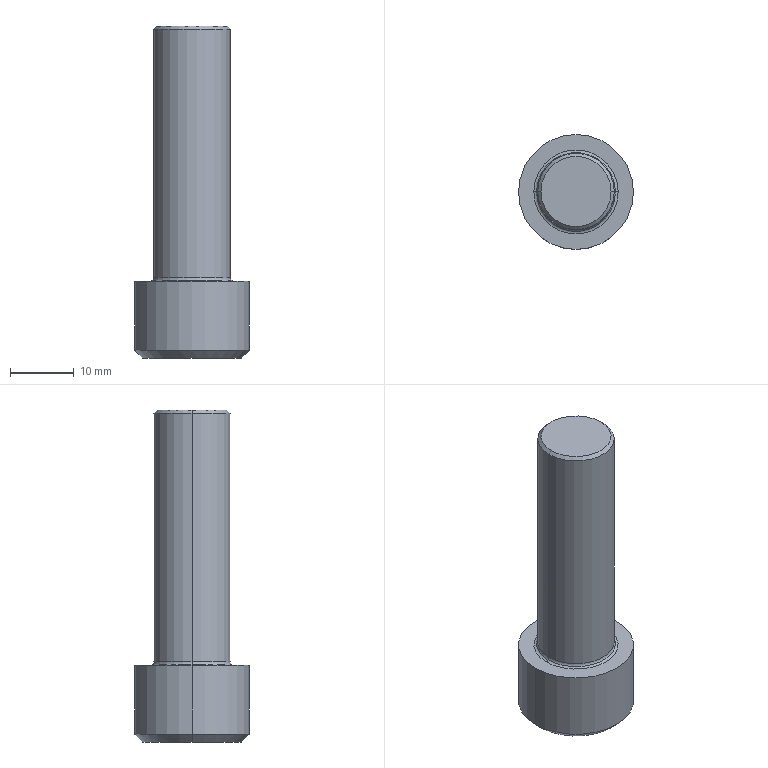Part | Creo | 1 solid | 23 faces | box 18 x 18 x 52 mm | volume 6904 mm3 | plane 9 | cone 6 | cylinder 4 | torus 4 | commonest cylinder face diameters 12 x2 18 x2
STEP:
#1=CARTESIAN_POINT('',(-0.7735,-90.005,-358.));
#2=VERTEX_POINT('',#1);
#3=CARTESIAN_POINT('',(2.113,-85.005,-358.));
#4=VERTEX_POINT('',#3);
#5=CARTESIAN_POINT('',(-0.7735,-90.005,-358.));
#6=CARTESIAN_POINT('',(-0.6388,-89.771,-357.922));
#7=CARTESIAN_POINT('',(-0.3685,-89.303,-357.782));
#8=CARTESIAN_POINT('',(0.04278,-88.591,-357.631));
#9=CARTESIAN_POINT('',(0.4589,-87.87,-357.55));
#10=CARTESIAN_POINT('',(0.8794,-87.142,-357.55));
#11=CARTESIAN_POINT('',(1.296,-86.42,-357.631));
#12=CARTESIAN_POINT('',(1.707,-85.709,-357.782));
#13=CARTESIAN_POINT('',(1.978,-85.239,-357.922));
#14=CARTESIAN_POINT('',(2.113,-85.005,-358.));
#15=B_SPLINE_CURVE_WITH_KNOTS('',3,(#5,#6,#7,#8,#9,#10,#11,#12,#13,#14),.UNSPECIFIED.,.F.,.F.,(4,1,1,1,1,1,1,4),(0.,0.1429,0.2857,0.4286,0.5714,0.7143,0.8571,1.),.UNSPECIFIED.);
#16=EDGE_CURVE('',#2,#4,#15,.T.);
#17=ORIENTED_EDGE('',*,*,#16,.F.);
#18=CARTESIAN_POINT('',(5.,-90.005,-354.667));
#19=VERTEX_POINT('',#18);
#20=CARTESIAN_POINT('',(5.,-90.005,-354.667));
#21=DIRECTION('',(-0.866,0.,-0.5));
#22=VECTOR('',#21,6.667);
#23=LINE('',#20,#22);
#24=EDGE_CURVE('',#19,#2,#23,.T.);
#25=ORIENTED_EDGE('',*,*,#24,.F.);
#26=CARTESIAN_POINT('',(10.774,-90.005,-358.));
#27=VERTEX_POINT('',#26);
#28=CARTESIAN_POINT('',(5.,-90.005,-354.667));
#29=DIRECTION('',(0.866,0.,-0.5));
#30=VECTOR('',#29,6.667);
#31=LINE('',#28,#30);
#32=EDGE_CURVE('',#19,#27,#31,.T.);
#33=ORIENTED_EDGE('',*,*,#32,.T.);
#34=CARTESIAN_POINT('',(7.887,-85.005,-358.));
#35=VERTEX_POINT('',#34);
#36=CARTESIAN_POINT('',(7.887,-85.005,-358.));
#37=CARTESIAN_POINT('',(8.021,-85.238,-357.922));
#38=CARTESIAN_POINT('',(8.292,-85.706,-357.782));
#39=CARTESIAN_POINT('',(8.703,-86.419,-357.631));
#40=CARTESIAN_POINT('',(9.119,-87.139,-357.55));
#41=CARTESIAN_POINT('',(9.54,-87.868,-357.55));
#42=CARTESIAN_POINT('',(9.956,-88.589,-357.631));
#43=CARTESIAN_POINT('',(10.367,-89.301,-357.782));
#44=CARTESIAN_POINT('',(10.638,-89.771,-357.922));
#45=CARTESIAN_POINT('',(10.774,-90.005,-358.));
#46=B_SPLINE_CURVE_WITH_KNOTS('',3,(#36,#37,#38,#39,#40,#41,#42,#43,#44,#45),.UNSPECIFIED.,.F.,.F.,(4,1,1,1,1,1,1,4),(0.,0.1429,0.2857,0.4286,0.5714,0.7143,0.8571,1.),.UNSPECIFIED.);
#47=EDGE_CURVE('',#35,#27,#46,.T.);
#48=ORIENTED_EDGE('',*,*,#47,.F.);
#49=CARTESIAN_POINT('',(2.113,-85.005,-358.));
#50=CARTESIAN_POINT('',(2.381,-85.005,-357.923));
#51=CARTESIAN_POINT('',(2.919,-85.005,-357.783));
#52=CARTESIAN_POINT('',(3.745,-85.005,-357.631));
#53=CARTESIAN_POINT('',(4.581,-85.005,-357.55));
#54=CARTESIAN_POINT('',(5.416,-85.005,-357.55));
#55=CARTESIAN_POINT('',(6.25,-85.005,-357.63));
#56=CARTESIAN_POINT('',(7.077,-85.005,-357.782));
#57=CARTESIAN_POINT('',(7.618,-85.005,-357.922));
#58=CARTESIAN_POINT('',(7.887,-85.005,-358.));
#59=B_SPLINE_CURVE_WITH_KNOTS('',3,(#49,#50,#51,#52,#53,#54,#55,#56,#57,#58),.UNSPECIFIED.,.F.,.F.,(4,1,1,1,1,1,1,4),(0.,0.1429,0.2857,0.4286,0.5714,0.7143,0.8571,1.),.UNSPECIFIED.);
#60=EDGE_CURVE('',#4,#35,#59,.T.);
#61=ORIENTED_EDGE('',*,*,#60,.F.);
#62=EDGE_LOOP('',(#17,#25,#33,#48,#61));
#63=FACE_OUTER_BOUND('',#62,.F.);
#64=CARTESIAN_POINT('',(5.,-90.005,-356.367));
#65=DIRECTION('',(0.,0.,-1.));
#66=DIRECTION('',(-1.,0.,0.));
#67=AXIS2_PLACEMENT_3D('',#64,#65,#66);
#68=CONICAL_SURFACE('',#67,2.944,60.);
#69=ADVANCED_FACE('',(#63),#68,.F.);
#70=CARTESIAN_POINT('',(2.113,-85.005,-364.));
#71=VERTEX_POINT('',#70);
#72=CARTESIAN_POINT('',(-0.7735,-90.005,-364.));
#73=VERTEX_POINT('',#72);
#74=CARTESIAN_POINT('',(2.113,-85.005,-364.));
#75=DIRECTION('',(-0.5,-0.866,0.));
#76=VECTOR('',#75,5.774);
#77=LINE('',#74,#76);
#78=EDGE_CURVE('',#71,#73,#77,.T.);
#79=ORIENTED_EDGE('',*,*,#78,.T.);
#80=CARTESIAN_POINT('',(-0.7735,-90.005,-364.));
#81=DIRECTION('',(0.,0.,1.));
#82=VECTOR('',#81,6.);
#83=LINE('',#80,#82);
#84=EDGE_CURVE('',#73,#2,#83,.T.);
#85=ORIENTED_EDGE('',*,*,#84,.T.);
#86=ORIENTED_EDGE('',*,*,#16,.T.);
#87=CARTESIAN_POINT('',(2.113,-85.005,-364.));
#88=DIRECTION('',(0.,0.,1.));
#89=VECTOR('',#88,6.);
#90=LINE('',#87,#89);
#91=EDGE_CURVE('',#71,#4,#90,.T.);
#92=ORIENTED_EDGE('',*,*,#91,.F.);
#93=EDGE_LOOP('',(#79,#85,#86,#92));
#94=FACE_OUTER_BOUND('',#93,.F.);
#95=CARTESIAN_POINT('',(2.113,-85.005,-358.));
#96=DIRECTION('',(0.866,-0.5,0.));
#97=DIRECTION('',(-0.5,-0.866,0.));
#98=AXIS2_PLACEMENT_3D('',#95,#96,#97);
#99=PLANE('',#98);
#100=ADVANCED_FACE('',(#94),#99,.T.);
#101=CARTESIAN_POINT('',(-2.8,-90.005,-364.));
#102=VERTEX_POINT('',#101);
#103=CARTESIAN_POINT('',(12.8,-90.005,-364.));
#104=VERTEX_POINT('',#103);
#105=CARTESIAN_POINT('',(5.,-90.005,-364.));
#106=DIRECTION('',(0.,0.,-1.));
#107=DIRECTION('',(-1.,0.,0.));
#108=AXIS2_PLACEMENT_3D('',#105,#106,#107);
#109=CIRCLE('',#108,7.8);
#110=EDGE_CURVE('',#102,#104,#109,.T.);
#111=ORIENTED_EDGE('',*,*,#110,.F.);
#112=CARTESIAN_POINT('',(5.,-90.005,-364.));
#113=DIRECTION('',(0.,0.,-1.));
#114=DIRECTION('',(1.,0.,0.));
#115=AXIS2_PLACEMENT_3D('',#112,#113,#114);
#116=CIRCLE('',#115,7.8);
#117=EDGE_CURVE('',#104,#102,#116,.T.);
#118=ORIENTED_EDGE('',*,*,#117,.F.);
#119=EDGE_LOOP('',(#111,#118));
#120=FACE_OUTER_BOUND('',#119,.F.);
#121=CARTESIAN_POINT('',(2.113,-95.005,-364.));
#122=VERTEX_POINT('',#121);
#123=CARTESIAN_POINT('',(-0.7735,-90.005,-364.));
#124=DIRECTION('',(0.5,-0.866,0.));
#125=VECTOR('',#124,5.774);
#126=LINE('',#123,#125);
#127=EDGE_CURVE('',#73,#122,#126,.T.);
#128=ORIENTED_EDGE('',*,*,#127,.F.);
#129=ORIENTED_EDGE('',*,*,#78,.F.);
#130=CARTESIAN_POINT('',(7.887,-85.005,-364.));
#131=VERTEX_POINT('',#130);
#132=CARTESIAN_POINT('',(2.113,-85.005,-364.));
#133=DIRECTION('',(1.,0.,0.));
#134=VECTOR('',#133,5.774);
#135=LINE('',#132,#134);
#136=EDGE_CURVE('',#71,#131,#135,.T.);
#137=ORIENTED_EDGE('',*,*,#136,.T.);
#138=CARTESIAN_POINT('',(10.774,-90.005,-364.));
#139=VERTEX_POINT('',#138);
#140=CARTESIAN_POINT('',(10.774,-90.005,-364.));
#141=DIRECTION('',(-0.5,0.866,0.));
#142=VECTOR('',#141,5.774);
#143=LINE('',#140,#142);
#144=EDGE_CURVE('',#139,#131,#143,.T.);
#145=ORIENTED_EDGE('',*,*,#144,.F.);
#146=CARTESIAN_POINT('',(7.887,-95.005,-364.));
#147=VERTEX_POINT('',#146);
#148=CARTESIAN_POINT('',(7.887,-95.005,-364.));
#149=DIRECTION('',(0.5,0.866,0.));
#150=VECTOR('',#149,5.774);
#151=LINE('',#148,#150);
#152=EDGE_CURVE('',#147,#139,#151,.T.);
#153=ORIENTED_EDGE('',*,*,#152,.F.);
#154=CARTESIAN_POINT('',(7.887,-95.005,-364.));
#155=DIRECTION('',(-1.,0.,0.));
#156=VECTOR('',#155,5.774);
#157=LINE('',#154,#156);
#158=EDGE_CURVE('',#147,#122,#157,.T.);
#159=ORIENTED_EDGE('',*,*,#158,.T.);
#160=EDGE_LOOP('',(#128,#129,#137,#145,#153,#159));
#161=FACE_BOUND('',#160,.F.);
#162=CARTESIAN_POINT('',(5.,-90.005,-364.));
#163=DIRECTION('',(0.,0.,-1.));
#164=DIRECTION('',(-1.,0.,0.));
#165=AXIS2_PLACEMENT_3D('',#162,#163,#164);
#166=PLANE('',#165);
#167=ADVANCED_FACE('',(#120,#161),#166,.T.);
#168=CARTESIAN_POINT('',(-4.,-90.005,-362.8));
#169=VERTEX_POINT('',#168);
#170=CARTESIAN_POINT('',(14.,-90.005,-362.8));
#171=VERTEX_POINT('',#170);
#172=CARTESIAN_POINT('',(5.,-90.005,-362.8));
#173=DIRECTION('',(0.,0.,-1.));
#174=DIRECTION('',(-1.,0.,0.));
#175=AXIS2_PLACEMENT_3D('',#172,#173,#174);
#176=CIRCLE('',#175,9.);
#177=EDGE_CURVE('',#169,#171,#176,.T.);
#178=ORIENTED_EDGE('',*,*,#177,.F.);
#179=CARTESIAN_POINT('',(-2.8,-90.005,-364.));
#180=DIRECTION('',(-0.7071,0.,0.7071));
#181=VECTOR('',#180,1.697);
#182=LINE('',#179,#181);
#183=EDGE_CURVE('',#102,#169,#182,.T.);
#184=ORIENTED_EDGE('',*,*,#183,.F.);
#185=ORIENTED_EDGE('',*,*,#110,.T.);
#186=CARTESIAN_POINT('',(12.8,-90.005,-364.));
#187=DIRECTION('',(0.7071,0.,0.7071));
#188=VECTOR('',#187,1.697);
#189=LINE('',#186,#188);
#190=EDGE_CURVE('',#104,#171,#189,.T.);
#191=ORIENTED_EDGE('',*,*,#190,.T.);
#192=EDGE_LOOP('',(#178,#184,#185,#191));
#193=FACE_OUTER_BOUND('',#192,.F.);
#194=CARTESIAN_POINT('',(5.,-90.005,-363.4));
#195=DIRECTION('',(0.,0.,1.));
#196=DIRECTION('',(1.,0.,0.));
#197=AXIS2_PLACEMENT_3D('',#194,#195,#196);
#198=CONICAL_SURFACE('',#197,8.4,45.);
#199=ADVANCED_FACE('',(#193),#198,.T.);
#200=ORIENTED_EDGE('',*,*,#177,.T.);
#201=CARTESIAN_POINT('',(14.,-90.005,-352.));
#202=VERTEX_POINT('',#201);
#203=CARTESIAN_POINT('',(14.,-90.005,-352.));
#204=DIRECTION('',(0.,0.,-1.));
#205=VECTOR('',#204,10.8);
#206=LINE('',#203,#205);
#207=EDGE_CURVE('',#202,#171,#206,.T.);
#208=ORIENTED_EDGE('',*,*,#207,.F.);
#209=CARTESIAN_POINT('',(-4.,-90.005,-352.));
#210=VERTEX_POINT('',#209);
#211=CARTESIAN_POINT('',(5.,-90.005,-352.));
#212=DIRECTION('',(0.,0.,1.));
#213=DIRECTION('',(1.,0.,0.));
#214=AXIS2_PLACEMENT_3D('',#211,#212,#213);
#215=CIRCLE('',#214,9.);
#216=EDGE_CURVE('',#202,#210,#215,.T.);
#217=ORIENTED_EDGE('',*,*,#216,.T.);
#218=CARTESIAN_POINT('',(-4.,-90.005,-352.));
#219=DIRECTION('',(0.,0.,-1.));
#220=VECTOR('',#219,10.8);
#221=LINE('',#218,#220);
#222=EDGE_CURVE('',#210,#169,#221,.T.);
#223=ORIENTED_EDGE('',*,*,#222,.T.);
#224=EDGE_LOOP('',(#200,#208,#217,#223));
#225=FACE_OUTER_BOUND('',#224,.F.);
#226=CARTESIAN_POINT('',(5.,-90.005,-352.));
#227=DIRECTION('',(0.,0.,-1.));
#228=DIRECTION('',(-1.,0.,0.));
#229=AXIS2_PLACEMENT_3D('',#226,#227,#228);
#230=CYLINDRICAL_SURFACE('',#229,9.);
#231=ADVANCED_FACE('',(#225),#230,.T.);
#232=CARTESIAN_POINT('',(5.,-90.005,-362.8));
#233=DIRECTION('',(0.,0.,-1.));
#234=DIRECTION('',(1.,0.,0.));
#235=AXIS2_PLACEMENT_3D('',#232,#233,#234);
#236=CIRCLE('',#235,9.);
#237=EDGE_CURVE('',#171,#169,#236,.T.);
#238=ORIENTED_EDGE('',*,*,#237,.T.);
#239=ORIENTED_EDGE('',*,*,#222,.F.);
#240=CARTESIAN_POINT('',(5.,-90.005,-352.));
#241=DIRECTION('',(0.,0.,1.));
#242=DIRECTION('',(-1.,0.,0.));
#243=AXIS2_PLACEMENT_3D('',#240,#241,#242);
#244=CIRCLE('',#243,9.);
#245=EDGE_CURVE('',#210,#202,#244,.T.);
#246=ORIENTED_EDGE('',*,*,#245,.T.);
#247=ORIENTED_EDGE('',*,*,#207,.T.);
#248=EDGE_LOOP('',(#238,#239,#246,#247));
#249=FACE_OUTER_BOUND('',#248,.F.);
#250=CARTESIAN_POINT('',(5.,-90.005,-352.));
#251=DIRECTION('',(0.,0.,-1.));
#252=DIRECTION('',(-1.,0.,0.));
#253=AXIS2_PLACEMENT_3D('',#250,#251,#252);
#254=CYLINDRICAL_SURFACE('',#253,9.);
#255=ADVANCED_FACE('',(#249),#254,.T.);
#256=ORIENTED_EDGE('',*,*,#237,.F.);
#257=ORIENTED_EDGE('',*,*,#190,.F.);
#258=ORIENTED_EDGE('',*,*,#117,.T.);
#259=ORIENTED_EDGE('',*,*,#183,.T.);
#260=EDGE_LOOP('',(#256,#257,#258,#259));
#261=FACE_OUTER_BOUND('',#260,.F.);
#262=CARTESIAN_POINT('',(5.,-90.005,-363.4));
#263=DIRECTION('',(0.,0.,1.));
#264=DIRECTION('',(1.,0.,0.));
#265=AXIS2_PLACEMENT_3D('',#262,#263,#264);
#266=CONICAL_SURFACE('',#265,8.4,45.);
#267=ADVANCED_FACE('',(#261),#266,.T.);
#268=ORIENTED_EDGE('',*,*,#245,.F.);
#269=ORIENTED_EDGE('',*,*,#216,.F.);
#270=EDGE_LOOP('',(#268,#269));
#271=FACE_OUTER_BOUND('',#270,.F.);
#272=CARTESIAN_POINT('',(-1.6,-90.005,-352.));
#273=VERTEX_POINT('',#272);
#274=CARTESIAN_POINT('',(11.6,-90.005,-352.));
#275=VERTEX_POINT('',#274);
#276=CARTESIAN_POINT('',(5.,-90.005,-352.));
#277=DIRECTION('',(0.,0.,-1.));
#278=DIRECTION('',(-1.,0.,0.));
#279=AXIS2_PLACEMENT_3D('',#276,#277,#278);
#280=CIRCLE('',#279,6.6);
#281=EDGE_CURVE('',#273,#275,#280,.T.);
#282=ORIENTED_EDGE('',*,*,#281,.F.);
#283=CARTESIAN_POINT('',(5.,-90.005,-352.));
#284=DIRECTION('',(0.,0.,-1.));
#285=DIRECTION('',(1.,0.,0.));
#286=AXIS2_PLACEMENT_3D('',#283,#284,#285);
#287=CIRCLE('',#286,6.6);
#288=EDGE_CURVE('',#275,#273,#287,.T.);
#289=ORIENTED_EDGE('',*,*,#288,.F.);
#290=EDGE_LOOP('',(#282,#289));
#291=FACE_BOUND('',#290,.F.);
#292=CARTESIAN_POINT('',(5.,-90.005,-352.));
#293=DIRECTION('',(0.,0.,-1.));
#294=DIRECTION('',(-1.,0.,0.));
#295=AXIS2_PLACEMENT_3D('',#292,#293,#294);
#296=PLANE('',#295);
#297=ADVANCED_FACE('',(#271,#291),#296,.F.);
#298=ORIENTED_EDGE('',*,*,#281,.T.);
#299=CARTESIAN_POINT('',(11.176,-90.005,-351.824));
#300=VERTEX_POINT('',#299);
#301=CARTESIAN_POINT('',(11.6,-90.005,-351.4));
#302=DIRECTION('',(0.,1.,0.));
#303=DIRECTION('',(0.,0.,-1.));
#304=AXIS2_PLACEMENT_3D('',#301,#302,#303);
#305=CIRCLE('',#304,0.6);
#306=EDGE_CURVE('',#275,#300,#305,.T.);
#307=ORIENTED_EDGE('',*,*,#306,.T.);
#308=CARTESIAN_POINT('',(-1.176,-90.005,-351.824));
#309=VERTEX_POINT('',#308);
#310=CARTESIAN_POINT('',(5.,-90.005,-351.824));
#311=DIRECTION('',(0.,0.,-1.));
#312=DIRECTION('',(-1.,0.,0.));
#313=AXIS2_PLACEMENT_3D('',#310,#311,#312);
#314=CIRCLE('',#313,6.176);
#315=EDGE_CURVE('',#309,#300,#314,.T.);
#316=ORIENTED_EDGE('',*,*,#315,.F.);
#317=CARTESIAN_POINT('',(-1.6,-90.005,-351.4));
#318=DIRECTION('',(0.,-1.,0.));
#319=DIRECTION('',(0.,0.,-1.));
#320=AXIS2_PLACEMENT_3D('',#317,#318,#319);
#321=CIRCLE('',#320,0.6);
#322=EDGE_CURVE('',#273,#309,#321,.T.);
#323=ORIENTED_EDGE('',*,*,#322,.F.);
#324=EDGE_LOOP('',(#298,#307,#316,#323));
#325=FACE_OUTER_BOUND('',#324,.F.);
#326=CARTESIAN_POINT('',(5.,-90.005,-351.4));
#327=DIRECTION('',(0.,0.,-1.));
#328=DIRECTION('',(-1.,0.,0.));
#329=AXIS2_PLACEMENT_3D('',#326,#327,#328);
#330=TOROIDAL_SURFACE('',#329,6.6,0.6);
#331=ADVANCED_FACE('',(#325),#330,.F.);
#332=ORIENTED_EDGE('',*,*,#288,.T.);
#333=ORIENTED_EDGE('',*,*,#322,.T.);
#334=CARTESIAN_POINT('',(5.,-90.005,-351.824));
#335=DIRECTION('',(0.,0.,-1.));
#336=DIRECTION('',(1.,0.,0.));
#337=AXIS2_PLACEMENT_3D('',#334,#335,#336);
#338=CIRCLE('',#337,6.176);
#339=EDGE_CURVE('',#300,#309,#338,.T.);
#340=ORIENTED_EDGE('',*,*,#339,.F.);
#341=ORIENTED_EDGE('',*,*,#306,.F.);
#342=EDGE_LOOP('',(#332,#333,#340,#341));
#343=FACE_OUTER_BOUND('',#342,.F.);
#344=CARTESIAN_POINT('',(5.,-90.005,-351.4));
#345=DIRECTION('',(0.,0.,-1.));
#346=DIRECTION('',(-1.,0.,0.));
#347=AXIS2_PLACEMENT_3D('',#344,#345,#346);
#348=TOROIDAL_SURFACE('',#347,6.6,0.6);
#349=ADVANCED_FACE('',(#343),#348,.F.);
#350=CARTESIAN_POINT('',(11.,-90.005,-351.4));
#351=VERTEX_POINT('',#350);
#352=CARTESIAN_POINT('',(-1.,-90.005,-351.4));
#353=VERTEX_POINT('',#352);
#354=CARTESIAN_POINT('',(5.,-90.005,-351.4));
#355=DIRECTION('',(0.,0.,-1.));
#356=DIRECTION('',(1.,0.,0.));
#357=AXIS2_PLACEMENT_3D('',#354,#355,#356);
#358=CIRCLE('',#357,6.);
#359=EDGE_CURVE('',#351,#353,#358,.T.);
#360=ORIENTED_EDGE('',*,*,#359,.F.);
#361=CARTESIAN_POINT('',(11.6,-90.005,-351.4));
#362=DIRECTION('',(0.,1.,0.));
#363=DIRECTION('',(-0.7071,0.,-0.7071));
#364=AXIS2_PLACEMENT_3D('',#361,#362,#363);
#365=CIRCLE('',#364,0.6);
#366=EDGE_CURVE('',#300,#351,#365,.T.);
#367=ORIENTED_EDGE('',*,*,#366,.F.);
#368=ORIENTED_EDGE('',*,*,#339,.T.);
#369=CARTESIAN_POINT('',(-1.6,-90.005,-351.4));
#370=DIRECTION('',(0.,-1.,0.));
#371=DIRECTION('',(0.7071,0.,-0.7071));
#372=AXIS2_PLACEMENT_3D('',#369,#370,#371);
#373=CIRCLE('',#372,0.6);
#374=EDGE_CURVE('',#309,#353,#373,.T.);
#375=ORIENTED_EDGE('',*,*,#374,.T.);
#376=EDGE_LOOP('',(#360,#367,#368,#375));
#377=FACE_OUTER_BOUND('',#376,.F.);
#378=CARTESIAN_POINT('',(5.,-90.005,-351.4));
#379=DIRECTION('',(0.,0.,-1.));
#380=DIRECTION('',(-1.,0.,0.));
#381=AXIS2_PLACEMENT_3D('',#378,#379,#380);
#382=TOROIDAL_SURFACE('',#381,6.6,0.6);
#383=ADVANCED_FACE('',(#377),#382,.F.);
#384=CARTESIAN_POINT('',(-1.,-90.005,-312.5));
#385=VERTEX_POINT('',#384);
#386=CARTESIAN_POINT('',(11.,-90.005,-312.5));
#387=VERTEX_POINT('',#386);
#388=CARTESIAN_POINT('',(5.,-90.005,-312.5));
#389=DIRECTION('',(0.,0.,1.));
#390=DIRECTION('',(-1.,0.,0.));
#391=AXIS2_PLACEMENT_3D('',#388,#389,#390);
#392=CIRCLE('',#391,6.);
#393=EDGE_CURVE('',#385,#387,#392,.T.);
#394=ORIENTED_EDGE('',*,*,#393,.T.);
#395=CARTESIAN_POINT('',(11.,-90.005,-312.5));
#396=DIRECTION('',(0.,0.,-1.));
#397=VECTOR('',#396,38.9);
#398=LINE('',#395,#397);
#399=EDGE_CURVE('',#387,#351,#398,.T.);
#400=ORIENTED_EDGE('',*,*,#399,.T.);
#401=ORIENTED_EDGE('',*,*,#359,.T.);
#402=CARTESIAN_POINT('',(-1.,-90.005,-312.5));
#403=DIRECTION('',(0.,0.,-1.));
#404=VECTOR('',#403,38.9);
#405=LINE('',#402,#404);
#406=EDGE_CURVE('',#385,#353,#405,.T.);
#407=ORIENTED_EDGE('',*,*,#406,.F.);
#408=EDGE_LOOP('',(#394,#400,#401,#407));
#409=FACE_OUTER_BOUND('',#408,.F.);
#410=CARTESIAN_POINT('',(5.,-90.005,-312.));
#411=DIRECTION('',(0.,0.,-1.));
#412=DIRECTION('',(-1.,0.,0.));
#413=AXIS2_PLACEMENT_3D('',#410,#411,#412);
#414=CYLINDRICAL_SURFACE('',#413,6.);
#415=ADVANCED_FACE('',(#409),#414,.T.);
#416=CARTESIAN_POINT('',(-0.5,-90.005,-312.));
#417=VERTEX_POINT('',#416);
#418=CARTESIAN_POINT('',(10.5,-90.005,-312.));
#419=VERTEX_POINT('',#418);
#420=CARTESIAN_POINT('',(5.,-90.005,-312.));
#421=DIRECTION('',(0.,0.,1.));
#422=DIRECTION('',(-1.,0.,0.));
#423=AXIS2_PLACEMENT_3D('',#420,#421,#422);
#424=CIRCLE('',#423,5.5);
#425=EDGE_CURVE('',#417,#419,#424,.T.);
#426=ORIENTED_EDGE('',*,*,#425,.T.);
#427=CARTESIAN_POINT('',(10.5,-90.005,-312.));
#428=DIRECTION('',(0.7071,0.,-0.7071));
#429=VECTOR('',#428,0.7071);
#430=LINE('',#427,#429);
#431=EDGE_CURVE('',#419,#387,#430,.T.);
#432=ORIENTED_EDGE('',*,*,#431,.T.);
#433=ORIENTED_EDGE('',*,*,#393,.F.);
#434=CARTESIAN_POINT('',(-0.5,-90.005,-312.));
#435=DIRECTION('',(-0.7071,0.,-0.7071));
#436=VECTOR('',#435,0.7071);
#437=LINE('',#434,#436);
#438=EDGE_CURVE('',#417,#385,#437,.T.);
#439=ORIENTED_EDGE('',*,*,#438,.F.);
#440=EDGE_LOOP('',(#426,#432,#433,#439));
#441=FACE_OUTER_BOUND('',#440,.F.);
#442=CARTESIAN_POINT('',(5.,-90.005,-312.25));
#443=DIRECTION('',(0.,0.,-1.));
#444=DIRECTION('',(-1.,0.,0.));
#445=AXIS2_PLACEMENT_3D('',#442,#443,#444);
#446=CONICAL_SURFACE('',#445,5.75,45.);
#447=ADVANCED_FACE('',(#441),#446,.T.);
#448=ORIENTED_EDGE('',*,*,#425,.F.);
#449=CARTESIAN_POINT('',(5.,-90.005,-312.));
#450=DIRECTION('',(0.,0.,1.));
#451=DIRECTION('',(1.,0.,0.));
#452=AXIS2_PLACEMENT_3D('',#449,#450,#451);
#453=CIRCLE('',#452,5.5);
#454=EDGE_CURVE('',#419,#417,#453,.T.);
#455=ORIENTED_EDGE('',*,*,#454,.F.);
#456=EDGE_LOOP('',(#448,#455));
#457=FACE_OUTER_BOUND('',#456,.F.);
#458=CARTESIAN_POINT('',(5.,-90.005,-312.));
#459=DIRECTION('',(0.,0.,-1.));
#460=DIRECTION('',(-1.,0.,0.));
#461=AXIS2_PLACEMENT_3D('',#458,#459,#460);
#462=PLANE('',#461);
#463=ADVANCED_FACE('',(#457),#462,.F.);
#464=ORIENTED_EDGE('',*,*,#454,.T.);
#465=ORIENTED_EDGE('',*,*,#438,.T.);
#466=CARTESIAN_POINT('',(5.,-90.005,-312.5));
#467=DIRECTION('',(0.,0.,1.));
#468=DIRECTION('',(1.,0.,0.));
#469=AXIS2_PLACEMENT_3D('',#466,#467,#468);
#470=CIRCLE('',#469,6.);
#471=EDGE_CURVE('',#387,#385,#470,.T.);
#472=ORIENTED_EDGE('',*,*,#471,.F.);
#473=ORIENTED_EDGE('',*,*,#431,.F.);
#474=EDGE_LOOP('',(#464,#465,#472,#473));
#475=FACE_OUTER_BOUND('',#474,.F.);
#476=CARTESIAN_POINT('',(5.,-90.005,-312.25));
#477=DIRECTION('',(0.,0.,-1.));
#478=DIRECTION('',(-1.,0.,0.));
#479=AXIS2_PLACEMENT_3D('',#476,#477,#478);
#480=CONICAL_SURFACE('',#479,5.75,45.);
#481=ADVANCED_FACE('',(#475),#480,.T.);
#482=ORIENTED_EDGE('',*,*,#471,.T.);
#483=ORIENTED_EDGE('',*,*,#406,.T.);
#484=CARTESIAN_POINT('',(5.,-90.005,-351.4));
#485=DIRECTION('',(0.,0.,-1.));
#486=DIRECTION('',(-1.,0.,0.));
#487=AXIS2_PLACEMENT_3D('',#484,#485,#486);
#488=CIRCLE('',#487,6.);
#489=EDGE_CURVE('',#353,#351,#488,.T.);
#490=ORIENTED_EDGE('',*,*,#489,.T.);
#491=ORIENTED_EDGE('',*,*,#399,.F.);
#492=EDGE_LOOP('',(#482,#483,#490,#491));
#493=FACE_OUTER_BOUND('',#492,.F.);
#494=CARTESIAN_POINT('',(5.,-90.005,-312.));
#495=DIRECTION('',(0.,0.,-1.));
#496=DIRECTION('',(-1.,0.,0.));
#497=AXIS2_PLACEMENT_3D('',#494,#495,#496);
#498=CYLINDRICAL_SURFACE('',#497,6.);
#499=ADVANCED_FACE('',(#493),#498,.T.);
#500=ORIENTED_EDGE('',*,*,#489,.F.);
#501=ORIENTED_EDGE('',*,*,#374,.F.);
#502=ORIENTED_EDGE('',*,*,#315,.T.);
#503=ORIENTED_EDGE('',*,*,#366,.T.);
#504=EDGE_LOOP('',(#500,#501,#502,#503));
#505=FACE_OUTER_BOUND('',#504,.F.);
#506=CARTESIAN_POINT('',(5.,-90.005,-351.4));
#507=DIRECTION('',(0.,0.,-1.));
#508=DIRECTION('',(-1.,0.,0.));
#509=AXIS2_PLACEMENT_3D('',#506,#507,#508);
#510=TOROIDAL_SURFACE('',#509,6.6,0.6);
#511=ADVANCED_FACE('',(#505),#510,.F.);
#512=ORIENTED_EDGE('',*,*,#127,.T.);
#513=CARTESIAN_POINT('',(2.113,-95.005,-358.));
#514=VERTEX_POINT('',#513);
#515=CARTESIAN_POINT('',(2.113,-95.005,-364.));
#516=DIRECTION('',(0.,0.,1.));
#517=VECTOR('',#516,6.);
#518=LINE('',#515,#517);
#519=EDGE_CURVE('',#122,#514,#518,.T.);
#520=ORIENTED_EDGE('',*,*,#519,.T.);
#521=CARTESIAN_POINT('',(2.113,-95.005,-358.));
#522=CARTESIAN_POINT('',(1.979,-94.771,-357.922));
#523=CARTESIAN_POINT('',(1.708,-94.303,-357.782));
#524=CARTESIAN_POINT('',(1.297,-93.591,-357.631));
#525=CARTESIAN_POINT('',(0.8808,-92.87,-357.55));
#526=CARTESIAN_POINT('',(0.4603,-92.142,-357.55));
#527=CARTESIAN_POINT('',(0.04376,-91.42,-357.631));
#528=CARTESIAN_POINT('',(-0.3671,-90.709,-357.782));
#529=CARTESIAN_POINT('',(-0.6383,-90.239,-357.922));
#530=CARTESIAN_POINT('',(-0.7735,-90.005,-358.));
#531=B_SPLINE_CURVE_WITH_KNOTS('',3,(#521,#522,#523,#524,#525,#526,#527,#528,#529,#530),.UNSPECIFIED.,.F.,.F.,(4,1,1,1,1,1,1,4),(0.,0.1429,0.2857,0.4286,0.5714,0.7143,0.8571,1.),.UNSPECIFIED.);
#532=EDGE_CURVE('',#514,#2,#531,.T.);
#533=ORIENTED_EDGE('',*,*,#532,.T.);
#534=ORIENTED_EDGE('',*,*,#84,.F.);
#535=EDGE_LOOP('',(#512,#520,#533,#534));
#536=FACE_OUTER_BOUND('',#535,.F.);
#537=CARTESIAN_POINT('',(-0.7735,-90.005,-358.));
#538=DIRECTION('',(0.866,0.5,0.));
#539=DIRECTION('',(0.5,-0.866,0.));
#540=AXIS2_PLACEMENT_3D('',#537,#538,#539);
#541=PLANE('',#540);
#542=ADVANCED_FACE('',(#536),#541,.T.);
#543=ORIENTED_EDGE('',*,*,#158,.F.);
#544=CARTESIAN_POINT('',(7.887,-95.005,-358.));
#545=VERTEX_POINT('',#544);
#546=CARTESIAN_POINT('',(7.887,-95.005,-364.));
#547=DIRECTION('',(0.,0.,1.));
#548=VECTOR('',#547,6.);
#549=LINE('',#546,#548);
#550=EDGE_CURVE('',#147,#545,#549,.T.);
#551=ORIENTED_EDGE('',*,*,#550,.T.);
#552=CARTESIAN_POINT('',(7.887,-95.005,-358.));
#553=CARTESIAN_POINT('',(7.618,-95.005,-357.922));
#554=CARTESIAN_POINT('',(7.077,-95.005,-357.782));
#555=CARTESIAN_POINT('',(6.25,-95.005,-357.63));
#556=CARTESIAN_POINT('',(5.416,-95.005,-357.55));
#557=CARTESIAN_POINT('',(4.581,-95.005,-357.55));
#558=CARTESIAN_POINT('',(3.745,-95.005,-357.631));
#559=CARTESIAN_POINT('',(2.919,-95.005,-357.783));
#560=CARTESIAN_POINT('',(2.381,-95.005,-357.923));
#561=CARTESIAN_POINT('',(2.113,-95.005,-358.));
#562=B_SPLINE_CURVE_WITH_KNOTS('',3,(#552,#553,#554,#555,#556,#557,#558,#559,#560,#561),.UNSPECIFIED.,.F.,.F.,(4,1,1,1,1,1,1,4),(0.,0.1429,0.2857,0.4286,0.5714,0.7143,0.8571,1.),.UNSPECIFIED.);
#563=EDGE_CURVE('',#545,#514,#562,.T.);
#564=ORIENTED_EDGE('',*,*,#563,.T.);
#565=ORIENTED_EDGE('',*,*,#519,.F.);
#566=EDGE_LOOP('',(#543,#551,#564,#565));
#567=FACE_OUTER_BOUND('',#566,.F.);
#568=CARTESIAN_POINT('',(2.113,-95.005,-358.));
#569=DIRECTION('',(0.,1.,0.));
#570=DIRECTION('',(0.,0.,-1.));
#571=AXIS2_PLACEMENT_3D('',#568,#569,#570);
#572=PLANE('',#571);
#573=ADVANCED_FACE('',(#567),#572,.T.);
#574=ORIENTED_EDGE('',*,*,#152,.T.);
#575=CARTESIAN_POINT('',(10.774,-90.005,-364.));
#576=DIRECTION('',(0.,0.,1.));
#577=VECTOR('',#576,6.);
#578=LINE('',#575,#577);
#579=EDGE_CURVE('',#139,#27,#578,.T.);
#580=ORIENTED_EDGE('',*,*,#579,.T.);
#581=CARTESIAN_POINT('',(10.774,-90.005,-358.));
#582=CARTESIAN_POINT('',(10.638,-90.239,-357.922));
#583=CARTESIAN_POINT('',(10.367,-90.709,-357.782));
#584=CARTESIAN_POINT('',(9.956,-91.42,-357.631));
#585=CARTESIAN_POINT('',(9.54,-92.142,-357.55));
#586=CARTESIAN_POINT('',(9.119,-92.87,-357.55));
#587=CARTESIAN_POINT('',(8.703,-93.591,-357.631));
#588=CARTESIAN_POINT('',(8.292,-94.303,-357.782));
#589=CARTESIAN_POINT('',(8.021,-94.771,-357.922));
#590=CARTESIAN_POINT('',(7.887,-95.005,-358.));
#591=B_SPLINE_CURVE_WITH_KNOTS('',3,(#581,#582,#583,#584,#585,#586,#587,#588,#589,#590),.UNSPECIFIED.,.F.,.F.,(4,1,1,1,1,1,1,4),(0.,0.1429,0.2857,0.4286,0.5714,0.7143,0.8571,1.),.UNSPECIFIED.);
#592=EDGE_CURVE('',#27,#545,#591,.T.);
#593=ORIENTED_EDGE('',*,*,#592,.T.);
#594=ORIENTED_EDGE('',*,*,#550,.F.);
#595=EDGE_LOOP('',(#574,#580,#593,#594));
#596=FACE_OUTER_BOUND('',#595,.F.);
#597=CARTESIAN_POINT('',(7.887,-95.005,-358.));
#598=DIRECTION('',(-0.866,0.5,0.));
#599=DIRECTION('',(0.5,0.866,0.));
#600=AXIS2_PLACEMENT_3D('',#597,#598,#599);
#601=PLANE('',#600);
#602=ADVANCED_FACE('',(#596),#601,.T.);
#603=ORIENTED_EDGE('',*,*,#144,.T.);
#604=CARTESIAN_POINT('',(7.887,-85.005,-364.));
#605=DIRECTION('',(0.,0.,1.));
#606=VECTOR('',#605,6.);
#607=LINE('',#604,#606);
#608=EDGE_CURVE('',#131,#35,#607,.T.);
#609=ORIENTED_EDGE('',*,*,#608,.T.);
#610=ORIENTED_EDGE('',*,*,#47,.T.);
#611=ORIENTED_EDGE('',*,*,#579,.F.);
#612=EDGE_LOOP('',(#603,#609,#610,#611));
#613=FACE_OUTER_BOUND('',#612,.F.);
#614=CARTESIAN_POINT('',(10.774,-90.005,-358.));
#615=DIRECTION('',(-0.866,-0.5,0.));
#616=DIRECTION('',(-0.5,0.866,0.));
#617=AXIS2_PLACEMENT_3D('',#614,#615,#616);
#618=PLANE('',#617);
#619=ADVANCED_FACE('',(#613),#618,.T.);
#620=ORIENTED_EDGE('',*,*,#136,.F.);
#621=ORIENTED_EDGE('',*,*,#91,.T.);
#622=ORIENTED_EDGE('',*,*,#60,.T.);
#623=ORIENTED_EDGE('',*,*,#608,.F.);
#624=EDGE_LOOP('',(#620,#621,#622,#623));
#625=FACE_OUTER_BOUND('',#624,.F.);
#626=CARTESIAN_POINT('',(7.887,-85.005,-358.));
#627=DIRECTION('',(0.,-1.,0.));
#628=DIRECTION('',(0.,0.,1.));
#629=AXIS2_PLACEMENT_3D('',#626,#627,#628);
#630=PLANE('',#629);
#631=ADVANCED_FACE('',(#625),#630,.T.);
#632=ORIENTED_EDGE('',*,*,#592,.F.);
#633=ORIENTED_EDGE('',*,*,#32,.F.);
#634=ORIENTED_EDGE('',*,*,#24,.T.);
#635=ORIENTED_EDGE('',*,*,#532,.F.);
#636=ORIENTED_EDGE('',*,*,#563,.F.);
#637=EDGE_LOOP('',(#632,#633,#634,#635,#636));
#638=FACE_OUTER_BOUND('',#637,.F.);
#639=CARTESIAN_POINT('',(5.,-90.005,-356.367));
#640=DIRECTION('',(0.,0.,-1.));
#641=DIRECTION('',(-1.,0.,0.));
#642=AXIS2_PLACEMENT_3D('',#639,#640,#641);
#643=CONICAL_SURFACE('',#642,2.944,60.);
#644=ADVANCED_FACE('',(#638),#643,.F.);
#645=CLOSED_SHELL('',(#69,#100,#167,#199,#231,#255,#267,#297,#331,#349,#383,#415,#447,#463,#481,#499,#511,#542,#573,#602,#619,#631,#644));
#646=MANIFOLD_SOLID_BREP('',#645);
#647=(LENGTH_UNIT()NAMED_UNIT(*)SI_UNIT(.MILLI.,.METRE.));
#648=UNCERTAINTY_MEASURE_WITH_UNIT(LENGTH_MEASURE(0.00579),#647,'','');
#649=(NAMED_UNIT(*)PLANE_ANGLE_UNIT()SI_UNIT($,.RADIAN.));
#650=PLANE_ANGLE_MEASURE_WITH_UNIT(PLANE_ANGLE_MEASURE(0.01745),#649);
#651=(CONVERSION_BASED_UNIT('DEGREE',#650)NAMED_UNIT(*)PLANE_ANGLE_UNIT());
#652=(NAMED_UNIT(*)SI_UNIT($,.STERADIAN.)SOLID_ANGLE_UNIT());
#653=(GEOMETRIC_REPRESENTATION_CONTEXT(3)GLOBAL_UNCERTAINTY_ASSIGNED_CONTEXT((#648))GLOBAL_UNIT_ASSIGNED_CONTEXT((#647,#651,#652))REPRESENTATION_CONTEXT('',''));
#654=ADVANCED_BREP_SHAPE_REPRESENTATION('',(#646),#653);